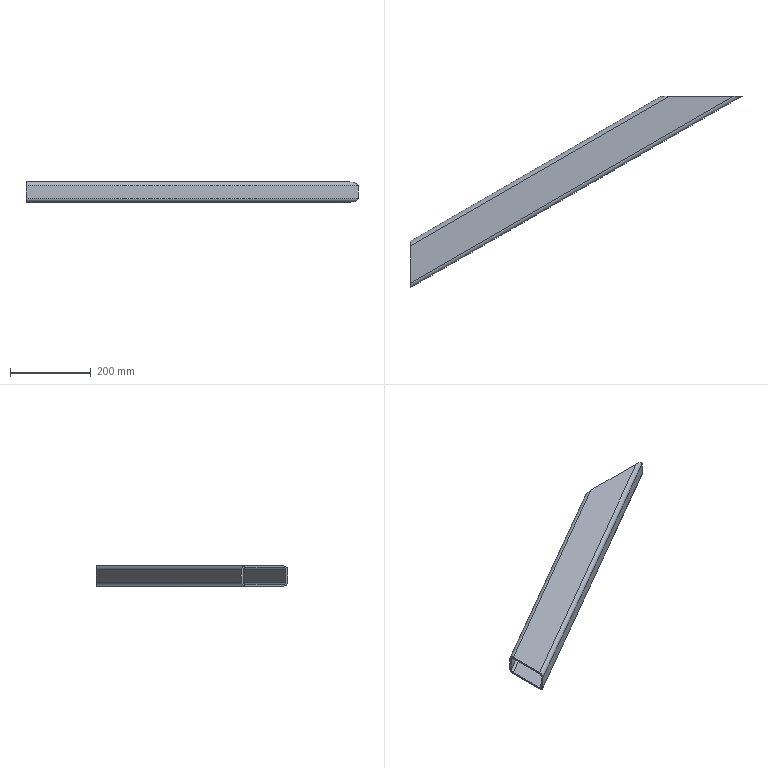Part | STEP file | Diagonal Brace矩形管-60度_Default<As Machined> | 1 solid | 18 faces | box 823.131 x 475.235 x 50 mm | volume 902687 mm3 | plane 10 | cylinder 8 | commonest cylinder face diameters 12 x4 20 x4